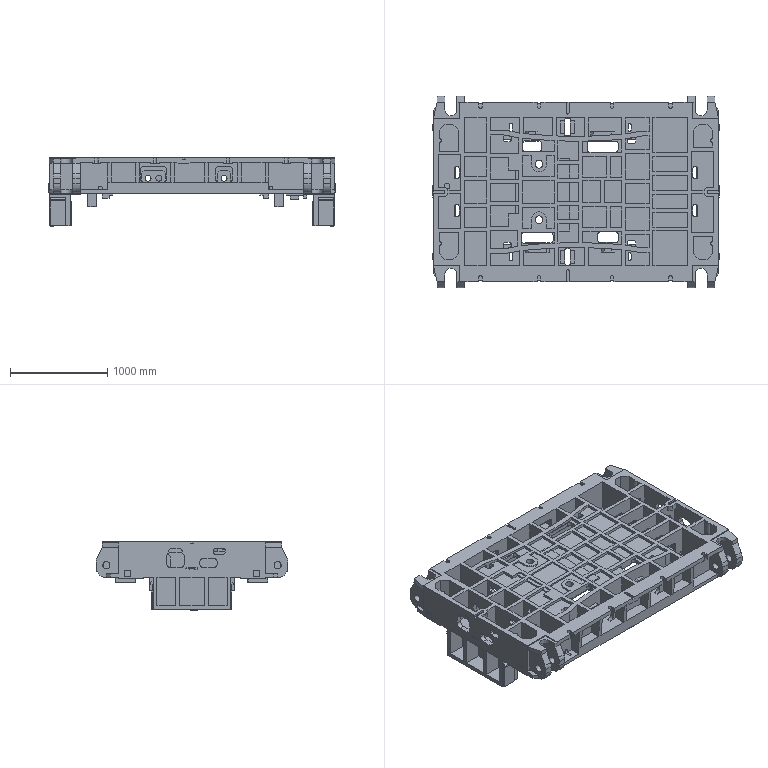Part | NX | features MAIN_BODY 2 | 1 solid | 1741 faces | box 2950 x 1970 x 700 mm | volume 684559551 mm3 | plane 1388 | cylinder 330 | spline 19 | cone 4 | commonest cylinder face diameters 80 x94 40 x76 60 x59 210 x16 50 x14 120 x12